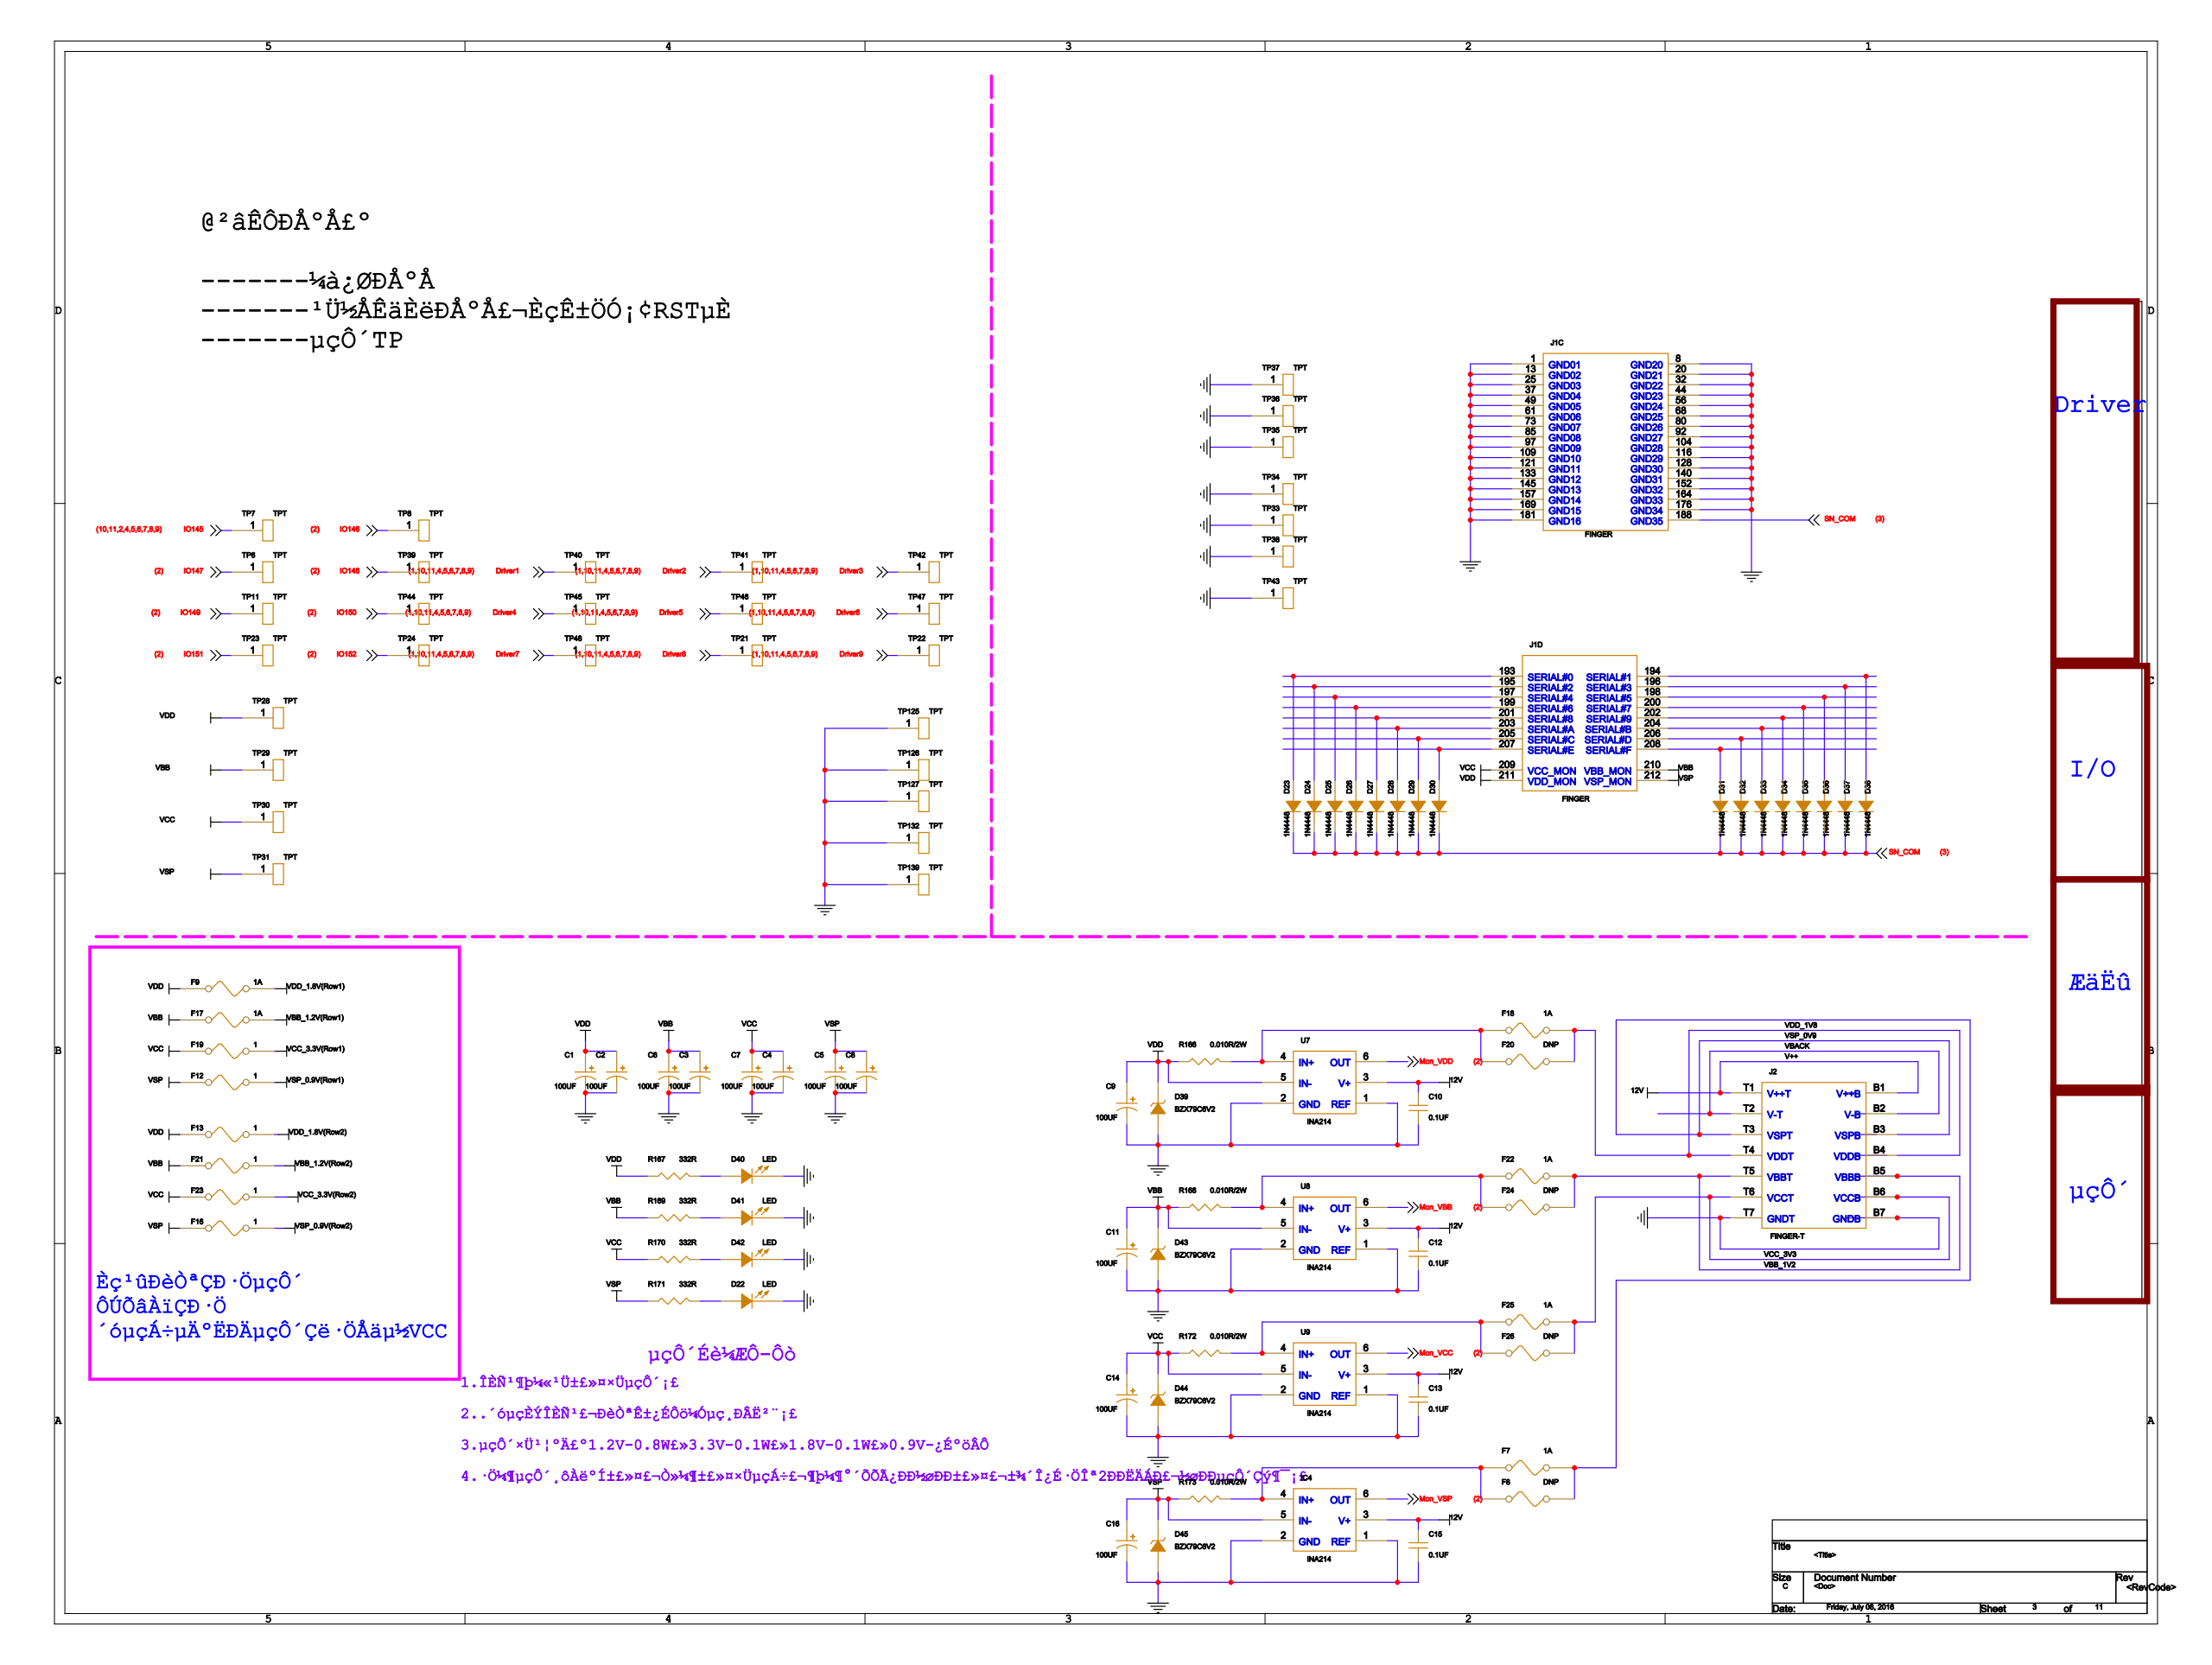Circuit board | Cadence Allegro | 531 parts | 624 nets | one sheet of the schematic
Parts on this sheet (reference | value | footprint):
C1 | 100UF | CAP2-1100
C2 | 100UF | CAP2-1100
C3 | 100UF | CAP2-1100
C4 | 100UF | CAP2-1100
C5 | 100UF | CAP2-1100
C6 | 100UF | CAP2-1100
C7 | 100UF | CAP2-1100
C8 | 100UF | CAP2-1100
C9 | 100UF | CAP2-1100
C10 | 0.1UF | C1206
C11 | 100UF | CAP2-1100
C12 | 0.1UF | C1206
C13 | 0.1UF | C1206
C14 | 100UF | CAP2-1100
C15 | 0.1UF | C1206
C16 | 100UF | CAP2-1100
D22 | LED | DIODE2-400
D23 | 1N4448 | DIODE2-400B
D24 | 1N4448 | DIODE2-400B
D25 | 1N4448 | DIODE2-400B
D26 | 1N4448 | DIODE2-400B
D27 | 1N4448 | DIODE2-400B
D28 | 1N4448 | DIODE2-400B
D29 | 1N4448 | DIODE2-400B
D30 | 1N4448 | DIODE2-400B
D31 | 1N4448 | DIODE2-400B
D32 | 1N4448 | DIODE2-400B
D33 | 1N4448 | DIODE2-400B
D34 | 1N4448 | DIODE2-400B
D35 | 1N4448 | DIODE2-400B
D36 | 1N4448 | DIODE2-400B
D37 | 1N4448 | DIODE2-400B
D38 | 1N4448 | DIODE2-400B
D39 | BZX79C6V2 | DIODE2-400B
D40 | LED | DIODE2-400
D41 | LED | DIODE2-400
D42 | LED | DIODE2-400
D43 | BZX79C6V2 | DIODE2-400B
D44 | BZX79C6V2 | DIODE2-400B
D45 | BZX79C6V2 | DIODE2-400B
F7 | 1A | FU2-600
F8 | DNP | FU2-600
F9 | 1A | FU2-600
F12 | 1 | FU2-600
F13 | 1 | FU2-600
F16 | 1 | FU2-600
F17 | 1A | FU2-600
F18 | 1A | FU2-600
F19 | 1 | FU2-600
F20 | DNP | FU2-600
F21 | 1 | FU2-600
F22 | 1A | FU2-600
F23 | 1 | FU2-600
F24 | DNP | FU2-600
F25 | 1A | FU2-600
F26 | DNP | FU2-600
IC4 | INA214 | SOP6-26-54
J1 | FINGER | FINGER
J2 | FINGER-T | FINGER-T
R166 | 0.010R/2W | R2512
R167 | 332R | R0805
R168 | 0.010R/2W | R2512
R169 | 332R | R0805
R170 | 332R | R0805
R171 | 332R | R0805
R172 | 0.010R/2W | R2512
R173 | 0.010R/2W | R2512
TP6 | TPT | TP36
TP7 | TPT | TP36
TP8 | TPT | TP36
TP11 | TPT | TP36
TP21 | TPT | TP36
TP22 | TPT | TP36
TP23 | TPT | TP36
TP24 | TPT | TP36
TP28 | TPT | TP36
TP29 | TPT | TP36
TP30 | TPT | TP36
TP31 | TPT | TP36
TP33 | TPT | TP36
TP34 | TPT | TP36
TP35 | TPT | TP36
TP36 | TPT | TP36
TP37 | TPT | TP36
TP38 | TPT | TP36
TP39 | TPT | TP36
TP40 | TPT | TP36
TP41 | TPT | TP36
TP42 | TPT | TP36
TP43 | TPT | TP36
TP44 | TPT | TP36
TP45 | TPT | TP36
TP46 | TPT | TP36
TP47 | TPT | TP36
TP48 | TPT | TP36
TP125 | TPT | TP36
TP126 | TPT | TP36
TP127 | TPT | TP36
TP132 | TPT | TP36
TP139 | TPT | TP36
U7 | INA214 | SOP6-26-54
U8 | INA214 | SOP6-26-54
U9 | INA214 | SOP6-26-54
Nets of these parts (net: part-pin ...):
GND: C1-2 C2-2 C3-2 C4-2 C5-2 C6-2 C7-2 C8-2 C9-2 C10-2 C11-2 C12-2 C13-2 C14-2 C15-2 C16-2 D22-2 D39-1 D40-2 D41-2 D42-2 D43-1 D44-1 D45-1 IC4-1 IC4-2 J2-B7 J2-T7 TP33-1 TP34-1 TP35-1 TP36-1 TP37-1 TP38-1 TP43-1 TP125-1 TP126-1 TP127-1 TP132-1 TP139-1 U7-1 U7-2 U8-1 U8-2 U9-1 U9-2 J1-1 J1-8 J1-13 J1-20 J1-25 J1-32 J1-37 J1-44 J1-49 J1-56 J1-61 J1-68 J1-73 J1-80 J1-85 J1-92 J1-97 J1-104 J1-109 J1-116 J1-121 J1-128 J1-133 J1-140 J1-145 J1-152 J1-157 J1-164 J1-169 J1-176 J1-181
VCC_3.3V(ROW1): F19-2
VCC_3.3V(ROW2): F23-2
N7809403: D22-1 R171-2
N390562: D40-1 R167-2
N393273: D41-1 R169-2
N393755: D42-1 R170-2
VDD: C1-1 C2-1 C9-1 D39-2 F9-1 F13-1 R166-1 R167-1 TP28-1 U7-5 J1-211
VBB: C3-1 C6-1 C11-1 D43-2 F17-1 F21-1 R168-1 R169-1 TP29-1 U8-5 J1-210
VCC: C4-1 C7-1 C14-1 D44-2 F19-1 F23-1 R170-1 R172-1 TP30-1 U9-5 J1-209
VSP: C5-1 C8-1 C16-1 D45-2 F12-1 F16-1 IC4-5 R171-1 R173-1 TP31-1 J1-212
VSP_0.9V(ROW1): F12-2
VDD_1.8V(ROW2): F13-2
VSP_0.9V(ROW2): F16-2
VBB_1.2V(ROW2): F21-2
VBB_1.2V(ROW1): F17-2
N321702: F18-1 F20-1 R166-2 U7-4
VDD_1V8: F18-2 F20-2 J2-B4 J2-T4
N326576: F22-1 F24-1 R168-2 U8-4
VBB_1V2: F22-2 F24-2 J2-B5 J2-T5
N327256: F25-1 F26-1 R172-2 U9-4
VCC_3V3: F25-2 F26-2 J2-B6 J2-T6
N7808239: F7-1 F8-1 IC4-4 R173-2
VSP_0V9: F7-2 F8-2 J2-B3 J2-T3
VDD_1.8V(ROW1): F9-2
IO145: TP7-1
DRIVER1: TP40-1
DRIVER3: TP42-1
DRIVER2: TP41-1
DRIVER4: TP45-1
DRIVER5: TP46-1
DRIVER6: TP47-1
DRIVER7: TP48-1
DRIVER8: TP21-1
DRIVER9: TP22-1
IO151: TP23-1
IO152: TP24-1
IO146: TP8-1
IO147: TP6-1
IO148: TP39-1
IO149: TP11-1
IO150: TP44-1
SN_COM: D23-2 D24-2 D25-2 D26-2 D27-2 D28-2 D29-2 D30-2 D31-2 D32-2 D33-2 D34-2 D35-2 D36-2 D37-2 D38-2 J1-188
MON_VSP: IC4-6
MON_VDD: U7-6
MON_VBB: U8-6
MON_VCC: U9-6
N423749: D23-1 J1-193
N431715: D38-1 J1-194
N424180: D24-1 J1-195
N431707: D37-1 J1-196
N424607: D25-1 J1-197
N431699: D36-1 J1-198
N425043: D26-1 J1-199
N431691: D35-1 J1-200
N425264: D27-1 J1-201
N431683: D34-1 J1-202
N425486: D28-1 J1-203
N431943: D33-1 J1-204
N425709: D29-1 J1-205
N431947: D32-1 J1-206
N425933: D30-1 J1-207
N431951: D31-1 J1-208
12V: C10-1 C12-1 C13-1 C15-1 IC4-3 J2-B1 J2-T1 U7-3 U8-3 U9-3
VBACK: J2-B2 J2-T2